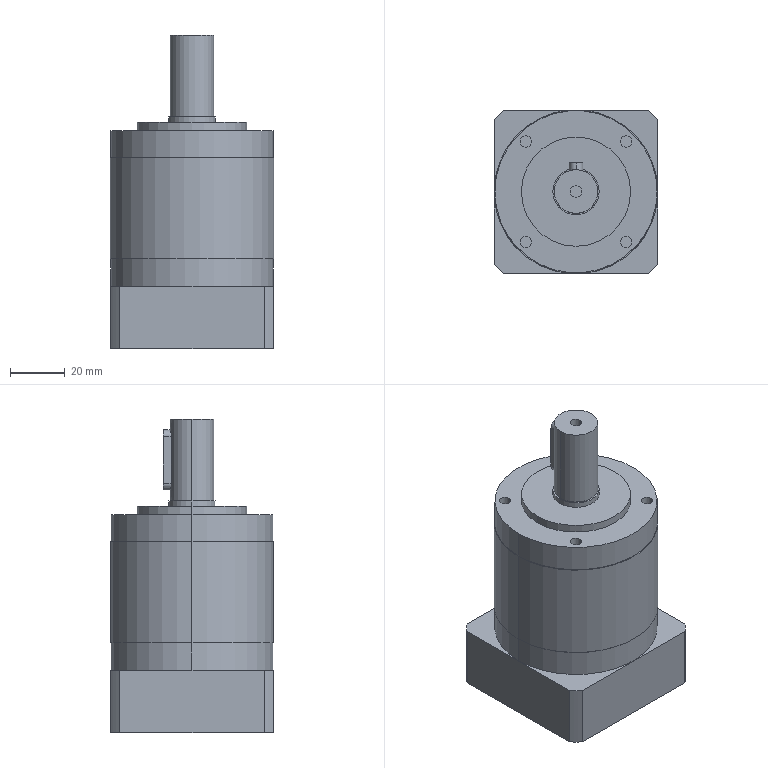Part | STEP file | Servo motor gearbox (PL60-8) | 1 solid | 67 faces | box 60 x 60 x 115 mm | volume 234745 mm3 | cylinder 41 | plane 26 | commonest cylinder face diameters 4.2 x18 59.4 x4 80 x4 5 x3 14 x2 16 x2